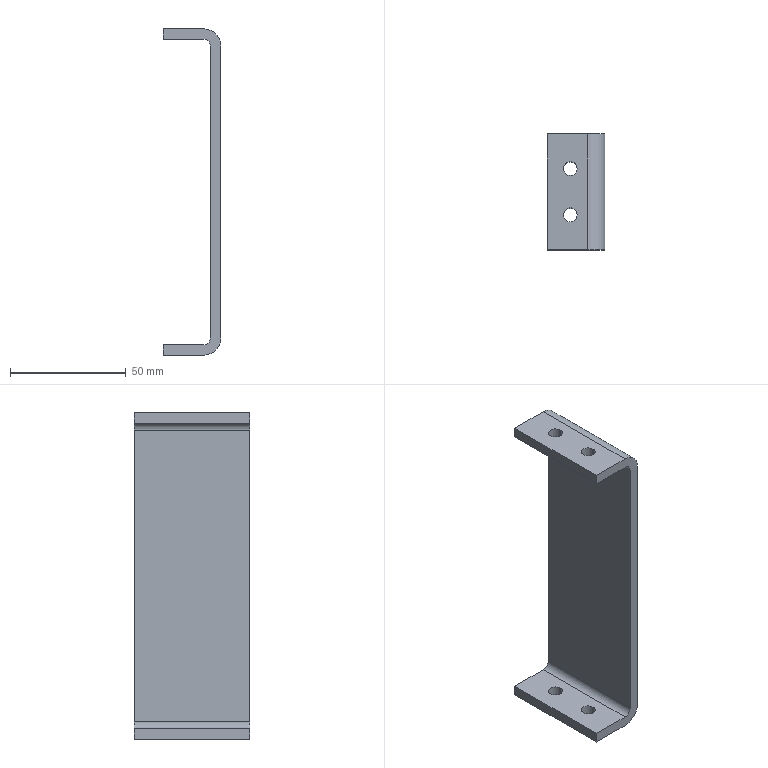Part | STEP file | END.BRACKET.1.stp | 1 solid | 22 faces | box 25 x 50 x 141 mm | volume 39427 mm3 | plane 10 | cylinder 8 | spline 4 | commonest cylinder face diameters 6 x6 15 x2